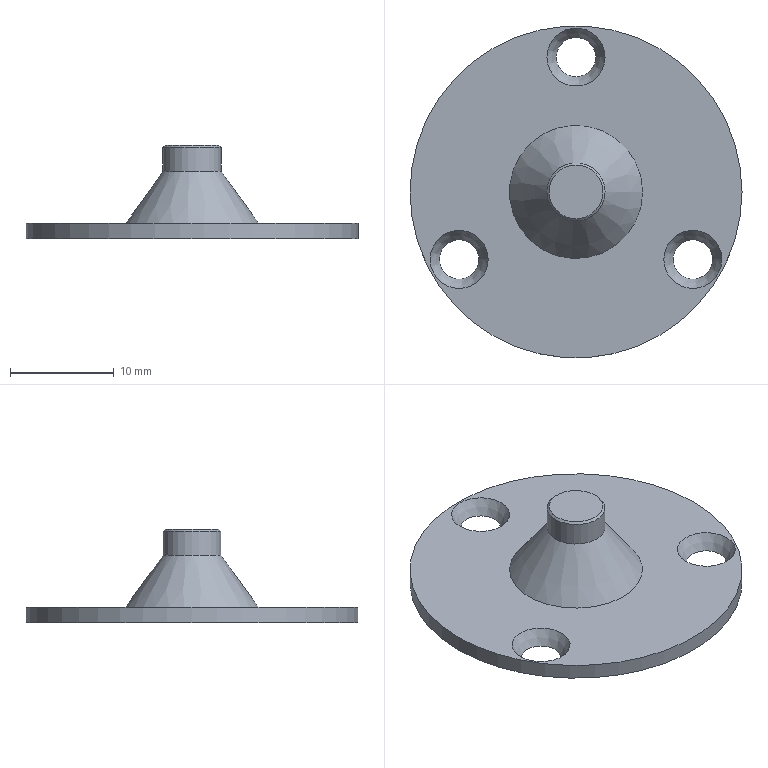Part | NX | 1 solid | 10 faces | box 32 x 32 x 9 mm | volume 1539 mm3 | cone 5 | plane 3 | cylinder 2 | commonest cylinder face diameters 5.6 x1 32 x1
STEP:
#1=CARTESIAN_POINT('',(-8.458,-6.5,1.5));
#2=VERTEX_POINT('',#1);
#3=CARTESIAN_POINT('',(-11.258,-6.5,1.5));
#4=DIRECTION('',(0.,0.,1.));
#5=DIRECTION('',(1.,0.,0.));
#6=AXIS2_PLACEMENT_3D('',#3,#4,#5);
#7=CIRCLE('',#6,2.8);
#8=EDGE_CURVE('',#2,#2,#7,.T.);
#9=ORIENTED_EDGE('',*,*,#8,.F.);
#10=EDGE_LOOP('',(#9));
#11=FACE_BOUND('',#10,.T.);
#12=CARTESIAN_POINT('',(6.415,0.,1.5));
#13=VERTEX_POINT('',#12);
#14=CARTESIAN_POINT('',(0.,0.,1.5));
#15=DIRECTION('',(0.,0.,1.));
#16=DIRECTION('',(1.,0.,0.));
#17=AXIS2_PLACEMENT_3D('',#14,#15,#16);
#18=CIRCLE('',#17,6.415);
#19=EDGE_CURVE('',#13,#13,#18,.F.);
#20=ORIENTED_EDGE('',*,*,#19,.T.);
#21=EDGE_LOOP('',(#20));
#22=FACE_BOUND('',#21,.T.);
#23=CARTESIAN_POINT('',(16.,0.,1.5));
#24=VERTEX_POINT('',#23);
#25=CARTESIAN_POINT('',(0.,0.,1.5));
#26=DIRECTION('',(0.,0.,1.));
#27=DIRECTION('',(1.,0.,0.));
#28=AXIS2_PLACEMENT_3D('',#25,#26,#27);
#29=CIRCLE('',#28,16.);
#30=EDGE_CURVE('',#24,#24,#29,.T.);
#31=ORIENTED_EDGE('',*,*,#30,.T.);
#32=EDGE_LOOP('',(#31));
#33=FACE_BOUND('',#32,.T.);
#34=CARTESIAN_POINT('',(2.8,13.,1.5));
#35=VERTEX_POINT('',#34);
#36=CARTESIAN_POINT('',(0.,13.,1.5));
#37=DIRECTION('',(0.,0.,1.));
#38=DIRECTION('',(1.,0.,0.));
#39=AXIS2_PLACEMENT_3D('',#36,#37,#38);
#40=CIRCLE('',#39,2.8);
#41=EDGE_CURVE('',#35,#35,#40,.T.);
#42=ORIENTED_EDGE('',*,*,#41,.F.);
#43=EDGE_LOOP('',(#42));
#44=FACE_BOUND('',#43,.T.);
#45=CARTESIAN_POINT('',(14.058,-6.5,1.5));
#46=VERTEX_POINT('',#45);
#47=CARTESIAN_POINT('',(11.258,-6.5,1.5));
#48=DIRECTION('',(0.,0.,1.));
#49=DIRECTION('',(1.,0.,0.));
#50=AXIS2_PLACEMENT_3D('',#47,#48,#49);
#51=CIRCLE('',#50,2.8);
#52=EDGE_CURVE('',#46,#46,#51,.T.);
#53=ORIENTED_EDGE('',*,*,#52,.F.);
#54=EDGE_LOOP('',(#53));
#55=FACE_BOUND('',#54,.T.);
#56=CARTESIAN_POINT('',(0.,0.,1.5));
#57=DIRECTION('',(0.,0.,1.));
#58=DIRECTION('',(1.,0.,0.));
#59=AXIS2_PLACEMENT_3D('',#56,#57,#58);
#60=PLANE('',#59);
#61=ADVANCED_FACE('',(#11,#22,#33,#44,#55),#60,.T.);
#62=CARTESIAN_POINT('',(-9.358,-6.5,0.));
#63=VERTEX_POINT('',#62);
#64=CARTESIAN_POINT('',(-11.258,-6.5,0.));
#65=DIRECTION('',(0.,0.,1.));
#66=DIRECTION('',(1.,0.,0.));
#67=AXIS2_PLACEMENT_3D('',#64,#65,#66);
#68=CIRCLE('',#67,1.9);
#69=EDGE_CURVE('',#63,#63,#68,.T.);
#70=ORIENTED_EDGE('',*,*,#69,.T.);
#71=EDGE_LOOP('',(#70));
#72=FACE_BOUND('',#71,.T.);
#73=CARTESIAN_POINT('',(16.,0.,0.));
#74=VERTEX_POINT('',#73);
#75=CARTESIAN_POINT('',(0.,0.,0.));
#76=DIRECTION('',(0.,0.,1.));
#77=DIRECTION('',(1.,0.,0.));
#78=AXIS2_PLACEMENT_3D('',#75,#76,#77);
#79=CIRCLE('',#78,16.);
#80=EDGE_CURVE('',#74,#74,#79,.T.);
#81=ORIENTED_EDGE('',*,*,#80,.F.);
#82=EDGE_LOOP('',(#81));
#83=FACE_BOUND('',#82,.T.);
#84=CARTESIAN_POINT('',(1.9,13.,0.));
#85=VERTEX_POINT('',#84);
#86=CARTESIAN_POINT('',(0.,13.,0.));
#87=DIRECTION('',(0.,0.,1.));
#88=DIRECTION('',(1.,0.,0.));
#89=AXIS2_PLACEMENT_3D('',#86,#87,#88);
#90=CIRCLE('',#89,1.9);
#91=EDGE_CURVE('',#85,#85,#90,.T.);
#92=ORIENTED_EDGE('',*,*,#91,.T.);
#93=EDGE_LOOP('',(#92));
#94=FACE_BOUND('',#93,.T.);
#95=CARTESIAN_POINT('',(13.158,-6.5,0.));
#96=VERTEX_POINT('',#95);
#97=CARTESIAN_POINT('',(11.258,-6.5,0.));
#98=DIRECTION('',(0.,0.,1.));
#99=DIRECTION('',(1.,0.,0.));
#100=AXIS2_PLACEMENT_3D('',#97,#98,#99);
#101=CIRCLE('',#100,1.9);
#102=EDGE_CURVE('',#96,#96,#101,.T.);
#103=ORIENTED_EDGE('',*,*,#102,.T.);
#104=EDGE_LOOP('',(#103));
#105=FACE_BOUND('',#104,.T.);
#106=CARTESIAN_POINT('',(0.,0.,0.));
#107=DIRECTION('',(0.,0.,1.));
#108=DIRECTION('',(1.,0.,0.));
#109=AXIS2_PLACEMENT_3D('',#106,#107,#108);
#110=PLANE('',#109);
#111=ADVANCED_FACE('',(#72,#83,#94,#105),#110,.F.);
#112=ORIENTED_EDGE('',*,*,#30,.F.);
#113=EDGE_LOOP('',(#112));
#114=FACE_BOUND('',#113,.T.);
#115=ORIENTED_EDGE('',*,*,#80,.T.);
#116=EDGE_LOOP('',(#115));
#117=FACE_BOUND('',#116,.T.);
#118=CARTESIAN_POINT('',(0.,0.,1.5));
#119=DIRECTION('',(0.,0.,-1.));
#120=DIRECTION('',(-1.,0.,0.));
#121=AXIS2_PLACEMENT_3D('',#118,#119,#120);
#122=CYLINDRICAL_SURFACE('',#121,16.);
#123=ADVANCED_FACE('',(#114,#117),#122,.T.);
#124=CARTESIAN_POINT('',(2.6,0.,9.));
#125=VERTEX_POINT('',#124);
#126=CARTESIAN_POINT('',(0.,0.,9.));
#127=DIRECTION('',(0.,0.,1.));
#128=DIRECTION('',(1.,0.,0.));
#129=AXIS2_PLACEMENT_3D('',#126,#127,#128);
#130=CIRCLE('',#129,2.6);
#131=EDGE_CURVE('',#125,#125,#130,.T.);
#132=ORIENTED_EDGE('',*,*,#131,.T.);
#133=EDGE_LOOP('',(#132));
#134=FACE_BOUND('',#133,.T.);
#135=CARTESIAN_POINT('',(0.,0.,9.));
#136=DIRECTION('',(0.,0.,-1.));
#137=DIRECTION('',(-1.,0.,0.));
#138=AXIS2_PLACEMENT_3D('',#135,#136,#137);
#139=PLANE('',#138);
#140=ADVANCED_FACE('',(#134),#139,.F.);
#141=ORIENTED_EDGE('',*,*,#131,.F.);
#142=EDGE_LOOP('',(#141));
#143=FACE_BOUND('',#142,.T.);
#144=CARTESIAN_POINT('',(2.8,0.,8.8));
#145=VERTEX_POINT('',#144);
#146=CARTESIAN_POINT('',(0.,0.,8.8));
#147=DIRECTION('',(0.,0.,1.));
#148=DIRECTION('',(1.,0.,0.));
#149=AXIS2_PLACEMENT_3D('',#146,#147,#148);
#150=CIRCLE('',#149,2.8);
#151=EDGE_CURVE('',#145,#145,#150,.T.);
#152=ORIENTED_EDGE('',*,*,#151,.T.);
#153=EDGE_LOOP('',(#152));
#154=FACE_BOUND('',#153,.T.);
#155=CARTESIAN_POINT('',(0.,0.,8.8));
#156=DIRECTION('',(0.,0.,-1.));
#157=DIRECTION('',(-1.,0.,0.));
#158=AXIS2_PLACEMENT_3D('',#155,#156,#157);
#159=CONICAL_SURFACE('',#158,2.8,0.7854);
#160=ADVANCED_FACE('',(#143,#154),#159,.T.);
#161=ORIENTED_EDGE('',*,*,#151,.F.);
#162=EDGE_LOOP('',(#161));
#163=FACE_BOUND('',#162,.T.);
#164=CARTESIAN_POINT('',(2.8,0.,6.5));
#165=VERTEX_POINT('',#164);
#166=CARTESIAN_POINT('',(0.,0.,6.5));
#167=DIRECTION('',(0.,0.,1.));
#168=DIRECTION('',(1.,0.,0.));
#169=AXIS2_PLACEMENT_3D('',#166,#167,#168);
#170=CIRCLE('',#169,2.8);
#171=EDGE_CURVE('',#165,#165,#170,.T.);
#172=ORIENTED_EDGE('',*,*,#171,.T.);
#173=EDGE_LOOP('',(#172));
#174=FACE_BOUND('',#173,.T.);
#175=CARTESIAN_POINT('',(0.,0.,0.));
#176=DIRECTION('',(0.,0.,1.));
#177=DIRECTION('',(1.,0.,0.));
#178=AXIS2_PLACEMENT_3D('',#175,#176,#177);
#179=CYLINDRICAL_SURFACE('',#178,2.8);
#180=ADVANCED_FACE('',(#163,#174),#179,.T.);
#181=ORIENTED_EDGE('',*,*,#19,.F.);
#182=EDGE_LOOP('',(#181));
#183=FACE_BOUND('',#182,.T.);
#184=ORIENTED_EDGE('',*,*,#171,.F.);
#185=EDGE_LOOP('',(#184));
#186=FACE_BOUND('',#185,.T.);
#187=CARTESIAN_POINT('',(0.,0.,0.));
#188=DIRECTION('',(0.,0.,-1.));
#189=DIRECTION('',(-1.,0.,0.));
#190=AXIS2_PLACEMENT_3D('',#187,#188,#189);
#191=CONICAL_SURFACE('',#190,7.5,0.626);
#192=ADVANCED_FACE('',(#183,#186),#191,.T.);
#193=ORIENTED_EDGE('',*,*,#41,.T.);
#194=EDGE_LOOP('',(#193));
#195=FACE_BOUND('',#194,.T.);
#196=ORIENTED_EDGE('',*,*,#91,.F.);
#197=EDGE_LOOP('',(#196));
#198=FACE_BOUND('',#197,.T.);
#199=CARTESIAN_POINT('',(0.,13.,0.));
#200=DIRECTION('',(0.,0.,1.));
#201=DIRECTION('',(1.,0.,0.));
#202=AXIS2_PLACEMENT_3D('',#199,#200,#201);
#203=CONICAL_SURFACE('',#202,1.9,0.5404);
#204=ADVANCED_FACE('',(#195,#198),#203,.F.);
#205=ORIENTED_EDGE('',*,*,#8,.T.);
#206=EDGE_LOOP('',(#205));
#207=FACE_BOUND('',#206,.T.);
#208=ORIENTED_EDGE('',*,*,#69,.F.);
#209=EDGE_LOOP('',(#208));
#210=FACE_BOUND('',#209,.T.);
#211=CARTESIAN_POINT('',(-11.258,-6.5,0.));
#212=DIRECTION('',(0.,0.,1.));
#213=DIRECTION('',(1.,0.,0.));
#214=AXIS2_PLACEMENT_3D('',#211,#212,#213);
#215=CONICAL_SURFACE('',#214,1.9,0.5404);
#216=ADVANCED_FACE('',(#207,#210),#215,.F.);
#217=ORIENTED_EDGE('',*,*,#52,.T.);
#218=EDGE_LOOP('',(#217));
#219=FACE_BOUND('',#218,.T.);
#220=ORIENTED_EDGE('',*,*,#102,.F.);
#221=EDGE_LOOP('',(#220));
#222=FACE_BOUND('',#221,.T.);
#223=CARTESIAN_POINT('',(11.258,-6.5,0.));
#224=DIRECTION('',(0.,0.,1.));
#225=DIRECTION('',(1.,0.,0.));
#226=AXIS2_PLACEMENT_3D('',#223,#224,#225);
#227=CONICAL_SURFACE('',#226,1.9,0.5404);
#228=ADVANCED_FACE('',(#219,#222),#227,.F.);
#229=CLOSED_SHELL('',(#61,#111,#123,#140,#160,#180,#192,#204,#216,#228));
#230=MANIFOLD_SOLID_BREP('',#229);
#231=(LENGTH_UNIT()NAMED_UNIT(*)SI_UNIT(.MILLI.,.METRE.));
#232=UNCERTAINTY_MEASURE_WITH_UNIT(LENGTH_MEASURE(0.00001),#231,'','');
#233=(NAMED_UNIT(*)PLANE_ANGLE_UNIT()SI_UNIT($,.RADIAN.));
#234=(NAMED_UNIT(*)SI_UNIT($,.STERADIAN.)SOLID_ANGLE_UNIT());
#235=(GEOMETRIC_REPRESENTATION_CONTEXT(3)GLOBAL_UNCERTAINTY_ASSIGNED_CONTEXT((#232))GLOBAL_UNIT_ASSIGNED_CONTEXT((#231,#233,#234))REPRESENTATION_CONTEXT('',''));
#236=ADVANCED_BREP_SHAPE_REPRESENTATION('',(#230),#235);